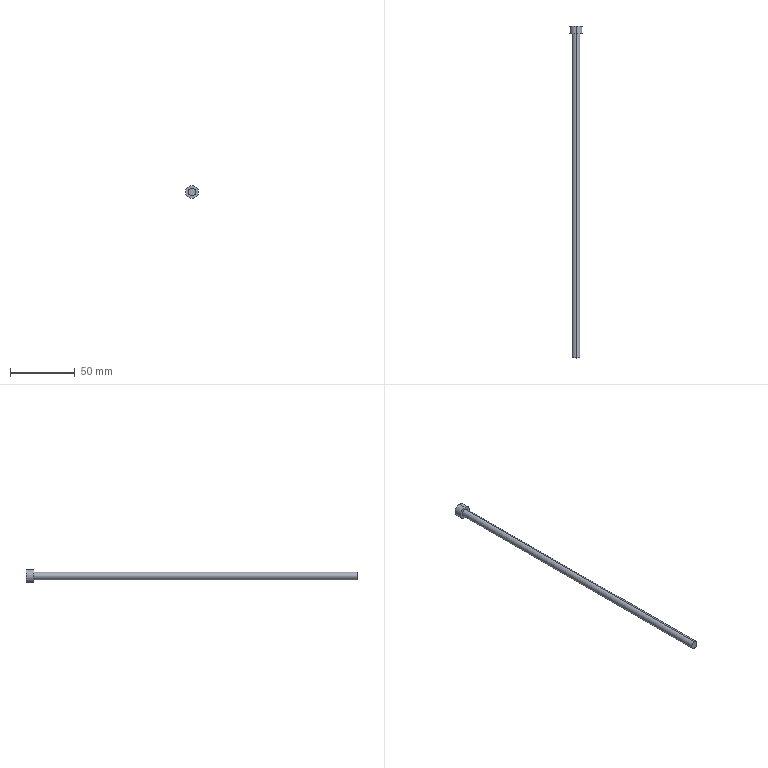Part | STEP file | 1 solid | 7 faces | box 10 x 257.335 x 10 mm | volume 7578 mm3 | cylinder 4 | plane 3 | commonest cylinder face diameters 6 x2 10 x2
STEP:
#1=CARTESIAN_POINT('',(0.,0.,0.));
#2=DIRECTION('',(0.,0.,1.));
#3=DIRECTION('',(1.,0.,0.));
#4=AXIS2_PLACEMENT_3D('',#1,#2,#3);
#5=CARTESIAN_POINT('',(-135.864,290.5,15.527));
#6=VERTEX_POINT('',#5);
#7=CARTESIAN_POINT('',(-135.864,290.5,25.527));
#8=VERTEX_POINT('',#7);
#9=CARTESIAN_POINT('',(-135.864,290.5,20.527));
#10=DIRECTION('',(0.,-1.,0.));
#11=DIRECTION('',(0.,0.,-1.));
#12=AXIS2_PLACEMENT_3D('',#9,#10,#11);
#13=CIRCLE('',#12,5.);
#14=CARTESIAN_POINT('',(-135.864,290.5,20.527));
#15=DIRECTION('',(0.,-1.,0.));
#16=DIRECTION('',(0.,0.,-1.));
#17=AXIS2_PLACEMENT_3D('',#14,#15,#16);
#18=CYLINDRICAL_SURFACE('',#17,5.);
#19=CARTESIAN_POINT('',(0.,0.));
#20=DIRECTION('',(1.,0.));
#21=VECTOR('',#20,1.);
#22=LINE('',#19,#21);
#23=(GEOMETRIC_REPRESENTATION_CONTEXT(2)PARAMETRIC_REPRESENTATION_CONTEXT()REPRESENTATION_CONTEXT('',''));
#24=DEFINITIONAL_REPRESENTATION('',(#22),#23);
#25=PCURVE('',#18,#24);
#26=CARTESIAN_POINT('',(-72.862,290.5,111.196));
#27=DIRECTION('',(0.,-1.,0.));
#28=DIRECTION('',(0.,0.,-1.));
#29=AXIS2_PLACEMENT_3D('',#26,#27,#28);
#30=PLANE('',#29);
#31=CARTESIAN_POINT('',(90.669,-63.002));
#32=DIRECTION('',(1.,0.));
#33=AXIS2_PLACEMENT_2D('',#31,#32);
#34=CIRCLE('',#33,5.);
#35=(GEOMETRIC_REPRESENTATION_CONTEXT(2)PARAMETRIC_REPRESENTATION_CONTEXT()REPRESENTATION_CONTEXT('',''));
#36=DEFINITIONAL_REPRESENTATION('',(#34),#35);
#37=PCURVE('',#30,#36);
#38=SURFACE_CURVE('',#13,(#25,#37),.PCURVE_S1.);
#39=EDGE_CURVE('',#6,#8,#38,.T.);
#40=ORIENTED_EDGE('',*,*,#39,.T.);
#41=CARTESIAN_POINT('',(-135.864,284.5,25.527));
#42=VERTEX_POINT('',#41);
#43=CARTESIAN_POINT('',(-135.864,290.5,25.527));
#44=DIRECTION('',(0.,-1.,0.));
#45=VECTOR('',#44,1.);
#46=LINE('',#43,#45);
#47=CARTESIAN_POINT('',(3.142,0.));
#48=DIRECTION('',(0.,1.));
#49=VECTOR('',#48,1.);
#50=LINE('',#47,#49);
#51=(GEOMETRIC_REPRESENTATION_CONTEXT(2)PARAMETRIC_REPRESENTATION_CONTEXT()REPRESENTATION_CONTEXT('',''));
#52=DEFINITIONAL_REPRESENTATION('',(#50),#51);
#53=PCURVE('',#18,#52);
#54=CARTESIAN_POINT('',(-135.864,290.5,20.527));
#55=DIRECTION('',(0.,-1.,0.));
#56=DIRECTION('',(0.,0.,-1.));
#57=AXIS2_PLACEMENT_3D('',#54,#55,#56);
#58=CYLINDRICAL_SURFACE('',#57,5.);
#59=CARTESIAN_POINT('',(3.142,0.));
#60=DIRECTION('',(0.,1.));
#61=VECTOR('',#60,1.);
#62=LINE('',#59,#61);
#63=(GEOMETRIC_REPRESENTATION_CONTEXT(2)PARAMETRIC_REPRESENTATION_CONTEXT()REPRESENTATION_CONTEXT('',''));
#64=DEFINITIONAL_REPRESENTATION('',(#62),#63);
#65=PCURVE('',#58,#64);
#66=SURFACE_CURVE('',#46,(#53,#65),.PCURVE_S1.);
#67=EDGE_CURVE('',#8,#42,#66,.T.);
#68=ORIENTED_EDGE('',*,*,#67,.T.);
#69=CARTESIAN_POINT('',(-135.864,284.5,15.527));
#70=VERTEX_POINT('',#69);
#71=CARTESIAN_POINT('',(-135.864,284.5,20.527));
#72=DIRECTION('',(0.,1.,0.));
#73=DIRECTION('',(0.,0.,1.));
#74=AXIS2_PLACEMENT_3D('',#71,#72,#73);
#75=CIRCLE('',#74,5.);
#76=CARTESIAN_POINT('',(3.142,6.));
#77=DIRECTION('',(-1.,0.));
#78=VECTOR('',#77,1.);
#79=LINE('',#76,#78);
#80=(GEOMETRIC_REPRESENTATION_CONTEXT(2)PARAMETRIC_REPRESENTATION_CONTEXT()REPRESENTATION_CONTEXT('',''));
#81=DEFINITIONAL_REPRESENTATION('',(#79),#80);
#82=PCURVE('',#18,#81);
#83=CARTESIAN_POINT('',(-135.864,284.5,20.527));
#84=DIRECTION('',(0.,-1.,0.));
#85=DIRECTION('',(0.,0.,-1.));
#86=AXIS2_PLACEMENT_3D('',#83,#84,#85);
#87=PLANE('',#86);
#88=CARTESIAN_POINT('',(-5.,0.));
#89=CARTESIAN_POINT('',(-5.,8.66));
#90=CARTESIAN_POINT('',(2.5,4.33));
#91=CARTESIAN_POINT('',(10.,0.));
#92=CARTESIAN_POINT('',(2.5,-4.33));
#93=CARTESIAN_POINT('',(-5.,-8.66));
#94=CARTESIAN_POINT('',(-5.,0.));
#95=(BOUNDED_CURVE()B_SPLINE_CURVE(2,(#88,#89,#90,#91,#92,#93,#94),.UNSPECIFIED.,.T.,.F.)B_SPLINE_CURVE_WITH_KNOTS((1,2,2,2,2,1),(-2.094,0.,2.094,4.189,6.283,8.378),.UNSPECIFIED.)CURVE()GEOMETRIC_REPRESENTATION_ITEM()RATIONAL_B_SPLINE_CURVE((1.,0.5,1.,0.5,1.,0.5,1.))REPRESENTATION_ITEM(''));
#96=(GEOMETRIC_REPRESENTATION_CONTEXT(2)PARAMETRIC_REPRESENTATION_CONTEXT()REPRESENTATION_CONTEXT('',''));
#97=DEFINITIONAL_REPRESENTATION('',(#95),#96);
#98=PCURVE('',#87,#97);
#99=SURFACE_CURVE('',#75,(#82,#98),.PCURVE_S1.);
#100=EDGE_CURVE('',#42,#70,#99,.T.);
#101=ORIENTED_EDGE('',*,*,#100,.T.);
#102=CARTESIAN_POINT('',(-135.864,290.5,15.527));
#103=DIRECTION('',(0.,-1.,0.));
#104=VECTOR('',#103,1.);
#105=LINE('',#102,#104);
#106=CARTESIAN_POINT('',(0.,0.));
#107=DIRECTION('',(0.,1.));
#108=VECTOR('',#107,1.);
#109=LINE('',#106,#108);
#110=(GEOMETRIC_REPRESENTATION_CONTEXT(2)PARAMETRIC_REPRESENTATION_CONTEXT()REPRESENTATION_CONTEXT('',''));
#111=DEFINITIONAL_REPRESENTATION('',(#109),#110);
#112=PCURVE('',#18,#111);
#113=CARTESIAN_POINT('',(6.283,0.));
#114=DIRECTION('',(0.,1.));
#115=VECTOR('',#114,1.);
#116=LINE('',#113,#115);
#117=(GEOMETRIC_REPRESENTATION_CONTEXT(2)PARAMETRIC_REPRESENTATION_CONTEXT()REPRESENTATION_CONTEXT('',''));
#118=DEFINITIONAL_REPRESENTATION('',(#116),#117);
#119=PCURVE('',#58,#118);
#120=SURFACE_CURVE('',#105,(#112,#119),.PCURVE_S1.);
#121=EDGE_CURVE('',#6,#70,#120,.T.);
#122=ORIENTED_EDGE('',*,*,#121,.F.);
#123=EDGE_LOOP('',(#40,#68,#101,#122));
#124=FACE_BOUND('',#123,.T.);
#125=ADVANCED_FACE('',(#124),#18,.T.);
#126=CARTESIAN_POINT('',(-135.864,284.5,23.527));
#127=VERTEX_POINT('',#126);
#128=CARTESIAN_POINT('',(-135.864,284.5,17.527));
#129=VERTEX_POINT('',#128);
#130=CARTESIAN_POINT('',(-135.864,284.5,20.527));
#131=DIRECTION('',(0.,1.,0.));
#132=DIRECTION('',(0.,0.,-1.));
#133=AXIS2_PLACEMENT_3D('',#130,#131,#132);
#134=CIRCLE('',#133,3.);
#135=CARTESIAN_POINT('',(-135.864,220.5,20.527));
#136=DIRECTION('',(0.,-1.,0.));
#137=DIRECTION('',(0.,0.,-1.));
#138=AXIS2_PLACEMENT_3D('',#135,#136,#137);
#139=CYLINDRICAL_SURFACE('',#138,3.);
#140=CARTESIAN_POINT('',(6.283,-64.));
#141=DIRECTION('',(-1.,0.));
#142=VECTOR('',#141,1.);
#143=LINE('',#140,#142);
#144=(GEOMETRIC_REPRESENTATION_CONTEXT(2)PARAMETRIC_REPRESENTATION_CONTEXT()REPRESENTATION_CONTEXT('',''));
#145=DEFINITIONAL_REPRESENTATION('',(#143),#144);
#146=PCURVE('',#139,#145);
#147=CARTESIAN_POINT('',(3.,0.));
#148=CARTESIAN_POINT('',(3.,-5.196));
#149=CARTESIAN_POINT('',(-1.5,-2.598));
#150=CARTESIAN_POINT('',(-6.,0.));
#151=CARTESIAN_POINT('',(-1.5,2.598));
#152=CARTESIAN_POINT('',(3.,5.196));
#153=CARTESIAN_POINT('',(3.,0.));
#154=(BOUNDED_CURVE()B_SPLINE_CURVE(2,(#147,#148,#149,#150,#151,#152,#153),.UNSPECIFIED.,.T.,.F.)B_SPLINE_CURVE_WITH_KNOTS((1,2,2,2,2,1),(-2.094,0.,2.094,4.189,6.283,8.378),.UNSPECIFIED.)CURVE()GEOMETRIC_REPRESENTATION_ITEM()RATIONAL_B_SPLINE_CURVE((1.,0.5,1.,0.5,1.,0.5,1.))REPRESENTATION_ITEM(''));
#155=(GEOMETRIC_REPRESENTATION_CONTEXT(2)PARAMETRIC_REPRESENTATION_CONTEXT()REPRESENTATION_CONTEXT('',''));
#156=DEFINITIONAL_REPRESENTATION('',(#154),#155);
#157=PCURVE('',#87,#156);
#158=SURFACE_CURVE('',#134,(#146,#157),.PCURVE_S1.);
#159=EDGE_CURVE('',#127,#129,#158,.T.);
#160=ORIENTED_EDGE('',*,*,#159,.F.);
#161=CARTESIAN_POINT('',(-135.864,33.165,23.527));
#162=VERTEX_POINT('',#161);
#163=CARTESIAN_POINT('',(-135.864,220.5,23.527));
#164=DIRECTION('',(0.,-1.,0.));
#165=VECTOR('',#164,1.);
#166=LINE('',#163,#165);
#167=CARTESIAN_POINT('',(3.142,0.));
#168=DIRECTION('',(0.,1.));
#169=VECTOR('',#168,1.);
#170=LINE('',#167,#169);
#171=(GEOMETRIC_REPRESENTATION_CONTEXT(2)PARAMETRIC_REPRESENTATION_CONTEXT()REPRESENTATION_CONTEXT('',''));
#172=DEFINITIONAL_REPRESENTATION('',(#170),#171);
#173=PCURVE('',#139,#172);
#174=CARTESIAN_POINT('',(-135.864,220.5,20.527));
#175=DIRECTION('',(0.,-1.,0.));
#176=DIRECTION('',(0.,0.,-1.));
#177=AXIS2_PLACEMENT_3D('',#174,#175,#176);
#178=CYLINDRICAL_SURFACE('',#177,3.);
#179=CARTESIAN_POINT('',(3.142,0.));
#180=DIRECTION('',(0.,1.));
#181=VECTOR('',#180,1.);
#182=LINE('',#179,#181);
#183=(GEOMETRIC_REPRESENTATION_CONTEXT(2)PARAMETRIC_REPRESENTATION_CONTEXT()REPRESENTATION_CONTEXT('',''));
#184=DEFINITIONAL_REPRESENTATION('',(#182),#183);
#185=PCURVE('',#178,#184);
#186=SURFACE_CURVE('',#166,(#173,#185),.PCURVE_S1.);
#187=EDGE_CURVE('',#127,#162,#186,.T.);
#188=ORIENTED_EDGE('',*,*,#187,.T.);
#189=CARTESIAN_POINT('',(-135.864,33.165,17.527));
#190=VERTEX_POINT('',#189);
#191=CARTESIAN_POINT('',(-135.864,33.165,20.527));
#192=DIRECTION('',(0.,1.,0.));
#193=DIRECTION('',(0.,0.,-1.));
#194=AXIS2_PLACEMENT_3D('',#191,#192,#193);
#195=CIRCLE('',#194,3.);
#196=CARTESIAN_POINT('',(6.283,187.335));
#197=DIRECTION('',(-1.,0.));
#198=VECTOR('',#197,1.);
#199=LINE('',#196,#198);
#200=(GEOMETRIC_REPRESENTATION_CONTEXT(2)PARAMETRIC_REPRESENTATION_CONTEXT()REPRESENTATION_CONTEXT('',''));
#201=DEFINITIONAL_REPRESENTATION('',(#199),#200);
#202=PCURVE('',#139,#201);
#203=CARTESIAN_POINT('',(-4.271,33.165,11.143));
#204=DIRECTION('',(0.,-1.,0.));
#205=DIRECTION('',(0.,0.,-1.));
#206=AXIS2_PLACEMENT_3D('',#203,#204,#205);
#207=PLANE('',#206);
#208=CARTESIAN_POINT('',(-6.384,-131.593));
#209=CARTESIAN_POINT('',(-6.384,-136.789));
#210=CARTESIAN_POINT('',(-10.884,-134.191));
#211=CARTESIAN_POINT('',(-15.384,-131.593));
#212=CARTESIAN_POINT('',(-10.884,-128.995));
#213=CARTESIAN_POINT('',(-6.384,-126.397));
#214=CARTESIAN_POINT('',(-6.384,-131.593));
#215=(BOUNDED_CURVE()B_SPLINE_CURVE(2,(#208,#209,#210,#211,#212,#213,#214),.UNSPECIFIED.,.T.,.F.)B_SPLINE_CURVE_WITH_KNOTS((1,2,2,2,2,1),(-2.094,0.,2.094,4.189,6.283,8.378),.UNSPECIFIED.)CURVE()GEOMETRIC_REPRESENTATION_ITEM()RATIONAL_B_SPLINE_CURVE((1.,0.5,1.,0.5,1.,0.5,1.))REPRESENTATION_ITEM(''));
#216=(GEOMETRIC_REPRESENTATION_CONTEXT(2)PARAMETRIC_REPRESENTATION_CONTEXT()REPRESENTATION_CONTEXT('',''));
#217=DEFINITIONAL_REPRESENTATION('',(#215),#216);
#218=PCURVE('',#207,#217);
#219=SURFACE_CURVE('',#195,(#202,#218),.PCURVE_S1.);
#220=EDGE_CURVE('',#162,#190,#219,.T.);
#221=ORIENTED_EDGE('',*,*,#220,.T.);
#222=CARTESIAN_POINT('',(-135.864,220.5,17.527));
#223=DIRECTION('',(0.,-1.,0.));
#224=VECTOR('',#223,1.);
#225=LINE('',#222,#224);
#226=CARTESIAN_POINT('',(0.,0.));
#227=DIRECTION('',(0.,1.));
#228=VECTOR('',#227,1.);
#229=LINE('',#226,#228);
#230=(GEOMETRIC_REPRESENTATION_CONTEXT(2)PARAMETRIC_REPRESENTATION_CONTEXT()REPRESENTATION_CONTEXT('',''));
#231=DEFINITIONAL_REPRESENTATION('',(#229),#230);
#232=PCURVE('',#139,#231);
#233=CARTESIAN_POINT('',(6.283,0.));
#234=DIRECTION('',(0.,1.));
#235=VECTOR('',#234,1.);
#236=LINE('',#233,#235);
#237=(GEOMETRIC_REPRESENTATION_CONTEXT(2)PARAMETRIC_REPRESENTATION_CONTEXT()REPRESENTATION_CONTEXT('',''));
#238=DEFINITIONAL_REPRESENTATION('',(#236),#237);
#239=PCURVE('',#178,#238);
#240=SURFACE_CURVE('',#225,(#232,#239),.PCURVE_S1.);
#241=EDGE_CURVE('',#129,#190,#240,.T.);
#242=ORIENTED_EDGE('',*,*,#241,.F.);
#243=EDGE_LOOP('',(#160,#188,#221,#242));
#244=FACE_BOUND('',#243,.T.);
#245=ADVANCED_FACE('',(#244),#139,.T.);
#246=ORIENTED_EDGE('',*,*,#187,.F.);
#247=CARTESIAN_POINT('',(-135.864,284.5,20.527));
#248=DIRECTION('',(0.,1.,0.));
#249=DIRECTION('',(0.,0.,-1.));
#250=AXIS2_PLACEMENT_3D('',#247,#248,#249);
#251=CIRCLE('',#250,3.);
#252=CARTESIAN_POINT('',(6.283,-64.));
#253=DIRECTION('',(-1.,0.));
#254=VECTOR('',#253,1.);
#255=LINE('',#252,#254);
#256=(GEOMETRIC_REPRESENTATION_CONTEXT(2)PARAMETRIC_REPRESENTATION_CONTEXT()REPRESENTATION_CONTEXT('',''));
#257=DEFINITIONAL_REPRESENTATION('',(#255),#256);
#258=PCURVE('',#178,#257);
#259=CARTESIAN_POINT('',(3.,0.));
#260=CARTESIAN_POINT('',(3.,-5.196));
#261=CARTESIAN_POINT('',(-1.5,-2.598));
#262=CARTESIAN_POINT('',(-6.,0.));
#263=CARTESIAN_POINT('',(-1.5,2.598));
#264=CARTESIAN_POINT('',(3.,5.196));
#265=CARTESIAN_POINT('',(3.,0.));
#266=(BOUNDED_CURVE()B_SPLINE_CURVE(2,(#259,#260,#261,#262,#263,#264,#265),.UNSPECIFIED.,.T.,.F.)B_SPLINE_CURVE_WITH_KNOTS((1,2,2,2,2,1),(-2.094,0.,2.094,4.189,6.283,8.378),.UNSPECIFIED.)CURVE()GEOMETRIC_REPRESENTATION_ITEM()RATIONAL_B_SPLINE_CURVE((1.,0.5,1.,0.5,1.,0.5,1.))REPRESENTATION_ITEM(''));
#267=(GEOMETRIC_REPRESENTATION_CONTEXT(2)PARAMETRIC_REPRESENTATION_CONTEXT()REPRESENTATION_CONTEXT('',''));
#268=DEFINITIONAL_REPRESENTATION('',(#266),#267);
#269=PCURVE('',#87,#268);
#270=SURFACE_CURVE('',#251,(#258,#269),.PCURVE_S1.);
#271=EDGE_CURVE('',#129,#127,#270,.T.);
#272=ORIENTED_EDGE('',*,*,#271,.F.);
#273=ORIENTED_EDGE('',*,*,#241,.T.);
#274=CARTESIAN_POINT('',(-135.864,33.165,20.527));
#275=DIRECTION('',(0.,1.,0.));
#276=DIRECTION('',(0.,0.,-1.));
#277=AXIS2_PLACEMENT_3D('',#274,#275,#276);
#278=CIRCLE('',#277,3.);
#279=CARTESIAN_POINT('',(6.283,187.335));
#280=DIRECTION('',(-1.,0.));
#281=VECTOR('',#280,1.);
#282=LINE('',#279,#281);
#283=(GEOMETRIC_REPRESENTATION_CONTEXT(2)PARAMETRIC_REPRESENTATION_CONTEXT()REPRESENTATION_CONTEXT('',''));
#284=DEFINITIONAL_REPRESENTATION('',(#282),#283);
#285=PCURVE('',#178,#284);
#286=CARTESIAN_POINT('',(-6.384,-131.593));
#287=CARTESIAN_POINT('',(-6.384,-136.789));
#288=CARTESIAN_POINT('',(-10.884,-134.191));
#289=CARTESIAN_POINT('',(-15.384,-131.593));
#290=CARTESIAN_POINT('',(-10.884,-128.995));
#291=CARTESIAN_POINT('',(-6.384,-126.397));
#292=CARTESIAN_POINT('',(-6.384,-131.593));
#293=(BOUNDED_CURVE()B_SPLINE_CURVE(2,(#286,#287,#288,#289,#290,#291,#292),.UNSPECIFIED.,.T.,.F.)B_SPLINE_CURVE_WITH_KNOTS((1,2,2,2,2,1),(-2.094,0.,2.094,4.189,6.283,8.378),.UNSPECIFIED.)CURVE()GEOMETRIC_REPRESENTATION_ITEM()RATIONAL_B_SPLINE_CURVE((1.,0.5,1.,0.5,1.,0.5,1.))REPRESENTATION_ITEM(''));
#294=(GEOMETRIC_REPRESENTATION_CONTEXT(2)PARAMETRIC_REPRESENTATION_CONTEXT()REPRESENTATION_CONTEXT('',''));
#295=DEFINITIONAL_REPRESENTATION('',(#293),#294);
#296=PCURVE('',#207,#295);
#297=SURFACE_CURVE('',#278,(#285,#296),.PCURVE_S1.);
#298=EDGE_CURVE('',#190,#162,#297,.T.);
#299=ORIENTED_EDGE('',*,*,#298,.T.);
#300=EDGE_LOOP('',(#246,#272,#273,#299));
#301=FACE_BOUND('',#300,.T.);
#302=ADVANCED_FACE('',(#301),#178,.T.);
#303=ORIENTED_EDGE('',*,*,#298,.F.);
#304=ORIENTED_EDGE('',*,*,#220,.F.);
#305=EDGE_LOOP('',(#303,#304));
#306=FACE_BOUND('',#305,.T.);
#307=ADVANCED_FACE('',(#306),#207,.T.);
#308=ORIENTED_EDGE('',*,*,#271,.T.);
#309=ORIENTED_EDGE('',*,*,#159,.T.);
#310=EDGE_LOOP('',(#308,#309));
#311=FACE_BOUND('',#310,.T.);
#312=CARTESIAN_POINT('',(-135.864,284.5,20.527));
#313=DIRECTION('',(0.,1.,0.));
#314=DIRECTION('',(0.,0.,1.));
#315=AXIS2_PLACEMENT_3D('',#312,#313,#314);
#316=CIRCLE('',#315,5.);
#317=CARTESIAN_POINT('',(-5.,0.));
#318=CARTESIAN_POINT('',(-5.,8.66));
#319=CARTESIAN_POINT('',(2.5,4.33));
#320=CARTESIAN_POINT('',(10.,0.));
#321=CARTESIAN_POINT('',(2.5,-4.33));
#322=CARTESIAN_POINT('',(-5.,-8.66));
#323=CARTESIAN_POINT('',(-5.,0.));
#324=(BOUNDED_CURVE()B_SPLINE_CURVE(2,(#317,#318,#319,#320,#321,#322,#323),.UNSPECIFIED.,.T.,.F.)B_SPLINE_CURVE_WITH_KNOTS((1,2,2,2,2,1),(-2.094,0.,2.094,4.189,6.283,8.378),.UNSPECIFIED.)CURVE()GEOMETRIC_REPRESENTATION_ITEM()RATIONAL_B_SPLINE_CURVE((1.,0.5,1.,0.5,1.,0.5,1.))REPRESENTATION_ITEM(''));
#325=(GEOMETRIC_REPRESENTATION_CONTEXT(2)PARAMETRIC_REPRESENTATION_CONTEXT()REPRESENTATION_CONTEXT('',''));
#326=DEFINITIONAL_REPRESENTATION('',(#324),#325);
#327=PCURVE('',#87,#326);
#328=CARTESIAN_POINT('',(9.425,6.));
#329=DIRECTION('',(-1.,0.));
#330=VECTOR('',#329,1.);
#331=LINE('',#328,#330);
#332=(GEOMETRIC_REPRESENTATION_CONTEXT(2)PARAMETRIC_REPRESENTATION_CONTEXT()REPRESENTATION_CONTEXT('',''));
#333=DEFINITIONAL_REPRESENTATION('',(#331),#332);
#334=PCURVE('',#58,#333);
#335=SURFACE_CURVE('',#316,(#327,#334),.PCURVE_S1.);
#336=EDGE_CURVE('',#70,#42,#335,.T.);
#337=ORIENTED_EDGE('',*,*,#336,.F.);
#338=ORIENTED_EDGE('',*,*,#100,.F.);
#339=EDGE_LOOP('',(#337,#338));
#340=FACE_BOUND('',#339,.T.);
#341=ADVANCED_FACE('',(#311,#340),#87,.T.);
#342=ORIENTED_EDGE('',*,*,#67,.F.);
#343=CARTESIAN_POINT('',(-135.864,290.5,20.527));
#344=DIRECTION('',(0.,-1.,0.));
#345=DIRECTION('',(0.,0.,-1.));
#346=AXIS2_PLACEMENT_3D('',#343,#344,#345);
#347=CIRCLE('',#346,5.);
#348=CARTESIAN_POINT('',(0.,0.));
#349=DIRECTION('',(1.,0.));
#350=VECTOR('',#349,1.);
#351=LINE('',#348,#350);
#352=(GEOMETRIC_REPRESENTATION_CONTEXT(2)PARAMETRIC_REPRESENTATION_CONTEXT()REPRESENTATION_CONTEXT('',''));
#353=DEFINITIONAL_REPRESENTATION('',(#351),#352);
#354=PCURVE('',#58,#353);
#355=CARTESIAN_POINT('',(90.669,-63.002));
#356=DIRECTION('',(1.,0.));
#357=AXIS2_PLACEMENT_2D('',#355,#356);
#358=CIRCLE('',#357,5.);
#359=(GEOMETRIC_REPRESENTATION_CONTEXT(2)PARAMETRIC_REPRESENTATION_CONTEXT()REPRESENTATION_CONTEXT('',''));
#360=DEFINITIONAL_REPRESENTATION('',(#358),#359);
#361=PCURVE('',#30,#360);
#362=SURFACE_CURVE('',#347,(#354,#361),.PCURVE_S1.);
#363=EDGE_CURVE('',#8,#6,#362,.T.);
#364=ORIENTED_EDGE('',*,*,#363,.T.);
#365=ORIENTED_EDGE('',*,*,#121,.T.);
#366=ORIENTED_EDGE('',*,*,#336,.T.);
#367=EDGE_LOOP('',(#342,#364,#365,#366));
#368=FACE_BOUND('',#367,.T.);
#369=ADVANCED_FACE('',(#368),#58,.T.);
#370=ORIENTED_EDGE('',*,*,#39,.F.);
#371=ORIENTED_EDGE('',*,*,#363,.F.);
#372=EDGE_LOOP('',(#370,#371));
#373=FACE_BOUND('',#372,.T.);
#374=ADVANCED_FACE('',(#373),#30,.F.);
#375=CLOSED_SHELL('',(#125,#245,#302,#307,#341,#369,#374));
#376=MANIFOLD_SOLID_BREP('',#375);
#377=(LENGTH_UNIT()NAMED_UNIT(*)SI_UNIT(.MILLI.,.METRE.));
#378=UNCERTAINTY_MEASURE_WITH_UNIT(LENGTH_MEASURE(0.0000001),#377,'','');
#379=(NAMED_UNIT(*)PLANE_ANGLE_UNIT()SI_UNIT($,.RADIAN.));
#380=(NAMED_UNIT(*)SI_UNIT($,.STERADIAN.)SOLID_ANGLE_UNIT());
#381=(GEOMETRIC_REPRESENTATION_CONTEXT(3)GLOBAL_UNCERTAINTY_ASSIGNED_CONTEXT((#378))GLOBAL_UNIT_ASSIGNED_CONTEXT((#377,#379,#380))REPRESENTATION_CONTEXT('',''));
#382=ADVANCED_BREP_SHAPE_REPRESENTATION('',(#4,#376),#381);